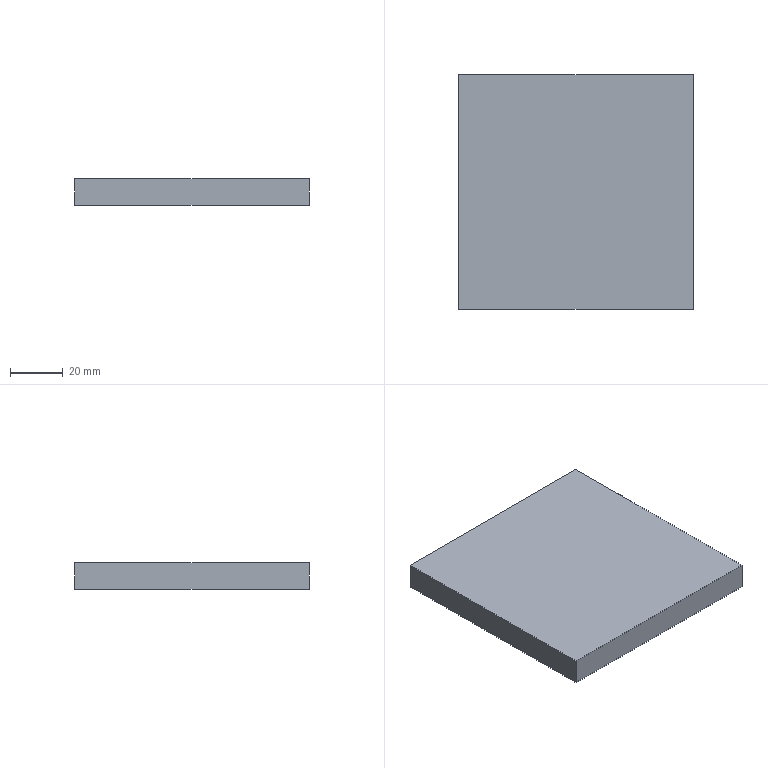Part | SolidWorks | features Extrusion 1 | 1 solid | 6 faces | box 88.9 x 88.9 x 10 mm | volume 79032 mm3 | plane 6
STEP:
#1=CARTESIAN_POINT('',(-44.45,44.45,-5.));
#2=VERTEX_POINT('',#1);
#3=CARTESIAN_POINT('',(-44.45,-44.45,-5.));
#4=VERTEX_POINT('',#3);
#5=CARTESIAN_POINT('',(-44.45,44.45,-5.));
#6=DIRECTION('',(0.,-1.,0.));
#7=VECTOR('',#6,1000.);
#8=LINE('',#5,#7);
#9=EDGE_CURVE('',#2,#4,#8,.T.);
#10=ORIENTED_EDGE('',*,*,#9,.T.);
#11=CARTESIAN_POINT('',(-44.45,-44.45,5.));
#12=VERTEX_POINT('',#11);
#13=CARTESIAN_POINT('',(-44.45,-44.45,5.));
#14=DIRECTION('',(0.,0.,-1.));
#15=VECTOR('',#14,1000.);
#16=LINE('',#13,#15);
#17=EDGE_CURVE('',#12,#4,#16,.T.);
#18=ORIENTED_EDGE('',*,*,#17,.F.);
#19=CARTESIAN_POINT('',(-44.45,44.45,5.));
#20=VERTEX_POINT('',#19);
#21=CARTESIAN_POINT('',(-44.45,44.45,5.));
#22=DIRECTION('',(0.,-1.,0.));
#23=VECTOR('',#22,1000.);
#24=LINE('',#21,#23);
#25=EDGE_CURVE('',#20,#12,#24,.T.);
#26=ORIENTED_EDGE('',*,*,#25,.F.);
#27=CARTESIAN_POINT('',(-44.45,44.45,5.));
#28=DIRECTION('',(0.,0.,-1.));
#29=VECTOR('',#28,1000.);
#30=LINE('',#27,#29);
#31=EDGE_CURVE('',#20,#2,#30,.T.);
#32=ORIENTED_EDGE('',*,*,#31,.T.);
#33=EDGE_LOOP('',(#10,#18,#26,#32));
#34=FACE_OUTER_BOUND('',#33,.T.);
#35=CARTESIAN_POINT('',(-44.45,44.45,5.));
#36=DIRECTION('',(1.,0.,0.));
#37=DIRECTION('',(0.,1.,0.));
#38=AXIS2_PLACEMENT_3D('',#35,#36,#37);
#39=PLANE('',#38);
#40=ADVANCED_FACE('',(#34),#39,.F.);
#41=CARTESIAN_POINT('',(44.45,-44.45,-5.));
#42=VERTEX_POINT('',#41);
#43=CARTESIAN_POINT('',(-44.45,-44.45,-5.));
#44=DIRECTION('',(1.,0.,0.));
#45=VECTOR('',#44,1000.);
#46=LINE('',#43,#45);
#47=EDGE_CURVE('',#4,#42,#46,.T.);
#48=ORIENTED_EDGE('',*,*,#47,.T.);
#49=CARTESIAN_POINT('',(44.45,-44.45,5.));
#50=VERTEX_POINT('',#49);
#51=CARTESIAN_POINT('',(44.45,-44.45,5.));
#52=DIRECTION('',(0.,0.,-1.));
#53=VECTOR('',#52,1000.);
#54=LINE('',#51,#53);
#55=EDGE_CURVE('',#50,#42,#54,.T.);
#56=ORIENTED_EDGE('',*,*,#55,.F.);
#57=CARTESIAN_POINT('',(-44.45,-44.45,5.));
#58=DIRECTION('',(1.,0.,0.));
#59=VECTOR('',#58,1000.);
#60=LINE('',#57,#59);
#61=EDGE_CURVE('',#12,#50,#60,.T.);
#62=ORIENTED_EDGE('',*,*,#61,.F.);
#63=ORIENTED_EDGE('',*,*,#17,.T.);
#64=EDGE_LOOP('',(#48,#56,#62,#63));
#65=FACE_OUTER_BOUND('',#64,.T.);
#66=CARTESIAN_POINT('',(-44.45,-44.45,5.));
#67=DIRECTION('',(0.,1.,0.));
#68=DIRECTION('',(0.,0.,1.));
#69=AXIS2_PLACEMENT_3D('',#66,#67,#68);
#70=PLANE('',#69);
#71=ADVANCED_FACE('',(#65),#70,.F.);
#72=CARTESIAN_POINT('',(44.45,44.45,-5.));
#73=VERTEX_POINT('',#72);
#74=CARTESIAN_POINT('',(44.45,44.45,-5.));
#75=DIRECTION('',(0.,1.,0.));
#76=VECTOR('',#75,1000.);
#77=LINE('',#74,#76);
#78=EDGE_CURVE('',#42,#73,#77,.T.);
#79=ORIENTED_EDGE('',*,*,#78,.T.);
#80=CARTESIAN_POINT('',(44.45,44.45,5.));
#81=VERTEX_POINT('',#80);
#82=CARTESIAN_POINT('',(44.45,44.45,5.));
#83=DIRECTION('',(0.,0.,-1.));
#84=VECTOR('',#83,1000.);
#85=LINE('',#82,#84);
#86=EDGE_CURVE('',#81,#73,#85,.T.);
#87=ORIENTED_EDGE('',*,*,#86,.F.);
#88=CARTESIAN_POINT('',(44.45,44.45,5.));
#89=DIRECTION('',(0.,1.,0.));
#90=VECTOR('',#89,1000.);
#91=LINE('',#88,#90);
#92=EDGE_CURVE('',#50,#81,#91,.T.);
#93=ORIENTED_EDGE('',*,*,#92,.F.);
#94=ORIENTED_EDGE('',*,*,#55,.T.);
#95=EDGE_LOOP('',(#79,#87,#93,#94));
#96=FACE_OUTER_BOUND('',#95,.T.);
#97=CARTESIAN_POINT('',(44.45,44.45,5.));
#98=DIRECTION('',(-1.,0.,0.));
#99=DIRECTION('',(0.,-1.,0.));
#100=AXIS2_PLACEMENT_3D('',#97,#98,#99);
#101=PLANE('',#100);
#102=ADVANCED_FACE('',(#96),#101,.F.);
#103=CARTESIAN_POINT('',(-44.45,44.45,-5.));
#104=DIRECTION('',(-1.,0.,0.));
#105=VECTOR('',#104,1000.);
#106=LINE('',#103,#105);
#107=EDGE_CURVE('',#73,#2,#106,.T.);
#108=ORIENTED_EDGE('',*,*,#107,.T.);
#109=ORIENTED_EDGE('',*,*,#31,.F.);
#110=CARTESIAN_POINT('',(-44.45,44.45,5.));
#111=DIRECTION('',(-1.,0.,0.));
#112=VECTOR('',#111,1000.);
#113=LINE('',#110,#112);
#114=EDGE_CURVE('',#81,#20,#113,.T.);
#115=ORIENTED_EDGE('',*,*,#114,.F.);
#116=ORIENTED_EDGE('',*,*,#86,.T.);
#117=EDGE_LOOP('',(#108,#109,#115,#116));
#118=FACE_OUTER_BOUND('',#117,.T.);
#119=CARTESIAN_POINT('',(-44.45,44.45,5.));
#120=DIRECTION('',(0.,-1.,0.));
#121=DIRECTION('',(1.,0.,0.));
#122=AXIS2_PLACEMENT_3D('',#119,#120,#121);
#123=PLANE('',#122);
#124=ADVANCED_FACE('',(#118),#123,.F.);
#125=ORIENTED_EDGE('',*,*,#25,.T.);
#126=ORIENTED_EDGE('',*,*,#61,.T.);
#127=ORIENTED_EDGE('',*,*,#92,.T.);
#128=ORIENTED_EDGE('',*,*,#114,.T.);
#129=EDGE_LOOP('',(#125,#126,#127,#128));
#130=FACE_OUTER_BOUND('',#129,.T.);
#131=CARTESIAN_POINT('',(0.,0.,5.));
#132=DIRECTION('',(0.,0.,1.));
#133=DIRECTION('',(1.,0.,0.));
#134=AXIS2_PLACEMENT_3D('',#131,#132,#133);
#135=PLANE('',#134);
#136=ADVANCED_FACE('',(#130),#135,.T.);
#137=ORIENTED_EDGE('',*,*,#9,.F.);
#138=ORIENTED_EDGE('',*,*,#107,.F.);
#139=ORIENTED_EDGE('',*,*,#78,.F.);
#140=ORIENTED_EDGE('',*,*,#47,.F.);
#141=EDGE_LOOP('',(#137,#138,#139,#140));
#142=FACE_OUTER_BOUND('',#141,.T.);
#143=CARTESIAN_POINT('',(0.,0.,-5.));
#144=DIRECTION('',(0.,0.,1.));
#145=DIRECTION('',(1.,0.,0.));
#146=AXIS2_PLACEMENT_3D('',#143,#144,#145);
#147=PLANE('',#146);
#148=ADVANCED_FACE('',(#142),#147,.F.);
#149=CLOSED_SHELL('',(#40,#71,#102,#124,#136,#148));
#150=MANIFOLD_SOLID_BREP('',#149);
#151=CARTESIAN_POINT('',(0.,0.,0.));
#152=DIRECTION('',(0.,0.,1.));
#153=DIRECTION('',(1.,0.,0.));
#154=AXIS2_PLACEMENT_3D('',#151,#152,#153);
#155=(LENGTH_UNIT()NAMED_UNIT(*)SI_UNIT(.MILLI.,.METRE.));
#156=UNCERTAINTY_MEASURE_WITH_UNIT(LENGTH_MEASURE(0.00001),#155,'','');
#157=(NAMED_UNIT(*)PLANE_ANGLE_UNIT()SI_UNIT($,.RADIAN.));
#158=(NAMED_UNIT(*)SI_UNIT($,.STERADIAN.)SOLID_ANGLE_UNIT());
#159=(GEOMETRIC_REPRESENTATION_CONTEXT(3)GLOBAL_UNCERTAINTY_ASSIGNED_CONTEXT((#156))GLOBAL_UNIT_ASSIGNED_CONTEXT((#155,#157,#158))REPRESENTATION_CONTEXT('',''));
#160=ADVANCED_BREP_SHAPE_REPRESENTATION('',(#150,#154),#159);